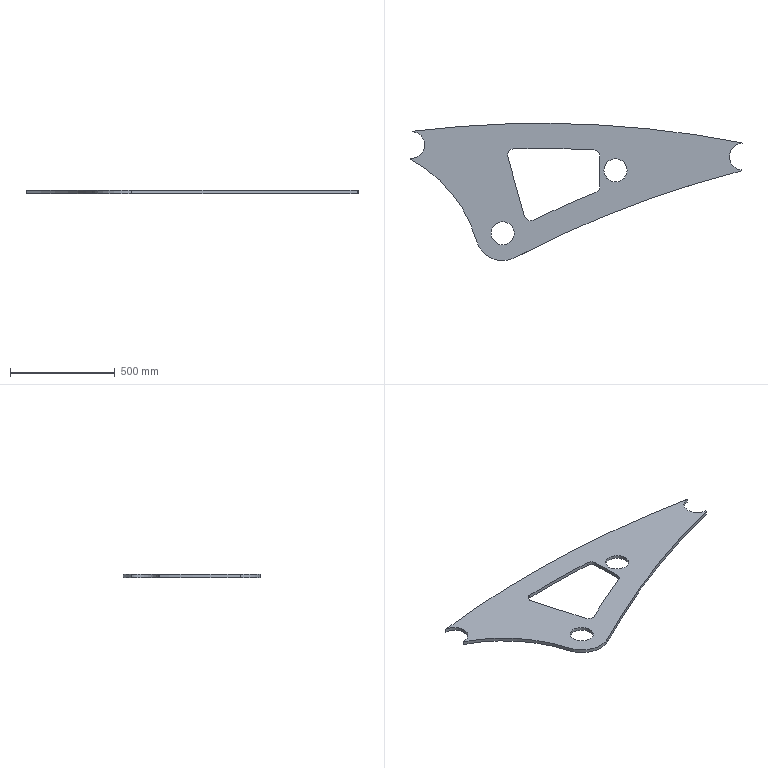Part | SolidWorks | features Extrusion 1 | 1 solid | 26 faces | box 1582 x 654.084 x 16 mm | volume 7594326 mm3 | cylinder 18 | plane 8 | commonest cylinder face diameters 60 x5 110 x4 128 x3 10000 x2 260 x1 1260 x1
STEP:
#1=CARTESIAN_POINT('',(52.281,402.337,16.));
#2=VERTEX_POINT('',#1);
#3=CARTESIAN_POINT('',(23.084,372.348,16.));
#4=VERTEX_POINT('',#3);
#5=CARTESIAN_POINT('',(53.084,372.348,16.));
#6=DIRECTION('',(0.,0.,1.));
#7=DIRECTION('',(-1.,0.,0.));
#8=AXIS2_PLACEMENT_3D('',#5,#6,#7);
#9=CIRCLE('',#8,30.);
#10=EDGE_CURVE('',#2,#4,#9,.T.);
#11=ORIENTED_EDGE('',*,*,#10,.T.);
#12=CARTESIAN_POINT('',(23.084,372.348,0.));
#13=VERTEX_POINT('',#12);
#14=CARTESIAN_POINT('',(23.084,372.348,16.));
#15=DIRECTION('',(0.,0.,-1.));
#16=VECTOR('',#15,1000.);
#17=LINE('',#14,#16);
#18=EDGE_CURVE('',#4,#13,#17,.T.);
#19=ORIENTED_EDGE('',*,*,#18,.T.);
#20=CARTESIAN_POINT('',(52.281,402.337,0.));
#21=VERTEX_POINT('',#20);
#22=CARTESIAN_POINT('',(53.084,372.348,0.));
#23=DIRECTION('',(0.,0.,1.));
#24=DIRECTION('',(-1.,0.,0.));
#25=AXIS2_PLACEMENT_3D('',#22,#23,#24);
#26=CIRCLE('',#25,30.);
#27=EDGE_CURVE('',#21,#13,#26,.T.);
#28=ORIENTED_EDGE('',*,*,#27,.F.);
#29=CARTESIAN_POINT('',(52.281,402.337,16.));
#30=DIRECTION('',(0.,0.,-1.));
#31=VECTOR('',#30,1000.);
#32=LINE('',#29,#31);
#33=EDGE_CURVE('',#2,#21,#32,.T.);
#34=ORIENTED_EDGE('',*,*,#33,.F.);
#35=EDGE_LOOP('',(#11,#19,#28,#34));
#36=FACE_OUTER_BOUND('',#35,.T.);
#37=CARTESIAN_POINT('',(53.084,372.348,16.));
#38=DIRECTION('',(0.,0.,-1.));
#39=DIRECTION('',(-1.,0.,0.));
#40=AXIS2_PLACEMENT_3D('',#37,#38,#39);
#41=CYLINDRICAL_SURFACE('',#40,30.);
#42=ADVANCED_FACE('',(#36),#41,.F.);
#43=CARTESIAN_POINT('',(483.,300.,16.));
#44=VERTEX_POINT('',#43);
#45=CARTESIAN_POINT('',(593.,300.,16.));
#46=VERTEX_POINT('',#45);
#47=CARTESIAN_POINT('',(538.,300.,16.));
#48=DIRECTION('',(0.,0.,1.));
#49=DIRECTION('',(1.,0.,0.));
#50=AXIS2_PLACEMENT_3D('',#47,#48,#49);
#51=CIRCLE('',#50,55.);
#52=EDGE_CURVE('',#44,#46,#51,.T.);
#53=ORIENTED_EDGE('',*,*,#52,.T.);
#54=CARTESIAN_POINT('',(593.,300.,0.));
#55=VERTEX_POINT('',#54);
#56=CARTESIAN_POINT('',(593.,300.,16.));
#57=DIRECTION('',(0.,0.,-1.));
#58=VECTOR('',#57,1000.);
#59=LINE('',#56,#58);
#60=EDGE_CURVE('',#46,#55,#59,.T.);
#61=ORIENTED_EDGE('',*,*,#60,.T.);
#62=CARTESIAN_POINT('',(483.,300.,0.));
#63=VERTEX_POINT('',#62);
#64=CARTESIAN_POINT('',(538.,300.,0.));
#65=DIRECTION('',(0.,0.,1.));
#66=DIRECTION('',(1.,0.,0.));
#67=AXIS2_PLACEMENT_3D('',#64,#65,#66);
#68=CIRCLE('',#67,55.);
#69=EDGE_CURVE('',#63,#55,#68,.T.);
#70=ORIENTED_EDGE('',*,*,#69,.F.);
#71=CARTESIAN_POINT('',(483.,300.,16.));
#72=DIRECTION('',(0.,0.,-1.));
#73=VECTOR('',#72,1000.);
#74=LINE('',#71,#73);
#75=EDGE_CURVE('',#44,#63,#74,.T.);
#76=ORIENTED_EDGE('',*,*,#75,.F.);
#77=EDGE_LOOP('',(#53,#61,#70,#76));
#78=FACE_OUTER_BOUND('',#77,.T.);
#79=CARTESIAN_POINT('',(538.,300.,16.));
#80=DIRECTION('',(0.,0.,-1.));
#81=DIRECTION('',(-1.,0.,0.));
#82=AXIS2_PLACEMENT_3D('',#79,#80,#81);
#83=CYLINDRICAL_SURFACE('',#82,55.);
#84=ADVANCED_FACE('',(#78),#83,.F.);
#85=CARTESIAN_POINT('',(-55.,0.,16.));
#86=VERTEX_POINT('',#85);
#87=CARTESIAN_POINT('',(55.,0.,16.));
#88=VERTEX_POINT('',#87);
#89=CARTESIAN_POINT('',(0.,0.,16.));
#90=DIRECTION('',(0.,0.,1.));
#91=DIRECTION('',(1.,0.,0.));
#92=AXIS2_PLACEMENT_3D('',#89,#90,#91);
#93=CIRCLE('',#92,55.);
#94=EDGE_CURVE('',#86,#88,#93,.T.);
#95=ORIENTED_EDGE('',*,*,#94,.T.);
#96=CARTESIAN_POINT('',(55.,0.,0.));
#97=VERTEX_POINT('',#96);
#98=CARTESIAN_POINT('',(55.,0.,16.));
#99=DIRECTION('',(0.,0.,-1.));
#100=VECTOR('',#99,1000.);
#101=LINE('',#98,#100);
#102=EDGE_CURVE('',#88,#97,#101,.T.);
#103=ORIENTED_EDGE('',*,*,#102,.T.);
#104=CARTESIAN_POINT('',(-55.,0.,0.));
#105=VERTEX_POINT('',#104);
#106=CARTESIAN_POINT('',(0.,0.,0.));
#107=DIRECTION('',(0.,0.,1.));
#108=DIRECTION('',(1.,0.,0.));
#109=AXIS2_PLACEMENT_3D('',#106,#107,#108);
#110=CIRCLE('',#109,55.);
#111=EDGE_CURVE('',#105,#97,#110,.T.);
#112=ORIENTED_EDGE('',*,*,#111,.F.);
#113=CARTESIAN_POINT('',(-55.,0.,16.));
#114=DIRECTION('',(0.,0.,-1.));
#115=VECTOR('',#114,1000.);
#116=LINE('',#113,#115);
#117=EDGE_CURVE('',#86,#105,#116,.T.);
#118=ORIENTED_EDGE('',*,*,#117,.F.);
#119=EDGE_LOOP('',(#95,#103,#112,#118));
#120=FACE_OUTER_BOUND('',#119,.T.);
#121=CARTESIAN_POINT('',(0.,0.,16.));
#122=DIRECTION('',(0.,0.,-1.));
#123=DIRECTION('',(-1.,0.,0.));
#124=AXIS2_PLACEMENT_3D('',#121,#122,#123);
#125=CYLINDRICAL_SURFACE('',#124,55.);
#126=ADVANCED_FACE('',(#120),#125,.F.);
#127=CARTESIAN_POINT('',(1080.5,365.5,16.));
#128=VERTEX_POINT('',#127);
#129=CARTESIAN_POINT('',(1140.709,429.388,16.));
#130=VERTEX_POINT('',#129);
#131=CARTESIAN_POINT('',(1144.5,365.5,16.));
#132=DIRECTION('',(0.,0.,-1.));
#133=DIRECTION('',(1.,0.,0.));
#134=AXIS2_PLACEMENT_3D('',#131,#132,#133);
#135=CIRCLE('',#134,64.);
#136=EDGE_CURVE('',#128,#130,#135,.T.);
#137=ORIENTED_EDGE('',*,*,#136,.F.);
#138=CARTESIAN_POINT('',(1080.5,365.5,0.));
#139=VERTEX_POINT('',#138);
#140=CARTESIAN_POINT('',(1080.5,365.5,16.));
#141=DIRECTION('',(0.,0.,-1.));
#142=VECTOR('',#141,1000.);
#143=LINE('',#140,#142);
#144=EDGE_CURVE('',#128,#139,#143,.T.);
#145=ORIENTED_EDGE('',*,*,#144,.T.);
#146=CARTESIAN_POINT('',(1140.709,429.388,0.));
#147=VERTEX_POINT('',#146);
#148=CARTESIAN_POINT('',(1144.5,365.5,0.));
#149=DIRECTION('',(0.,0.,-1.));
#150=DIRECTION('',(1.,0.,0.));
#151=AXIS2_PLACEMENT_3D('',#148,#149,#150);
#152=CIRCLE('',#151,64.);
#153=EDGE_CURVE('',#139,#147,#152,.T.);
#154=ORIENTED_EDGE('',*,*,#153,.T.);
#155=CARTESIAN_POINT('',(1140.709,429.388,16.));
#156=DIRECTION('',(0.,0.,-1.));
#157=VECTOR('',#156,1000.);
#158=LINE('',#155,#157);
#159=EDGE_CURVE('',#130,#147,#158,.T.);
#160=ORIENTED_EDGE('',*,*,#159,.F.);
#161=EDGE_LOOP('',(#137,#145,#154,#160));
#162=FACE_OUTER_BOUND('',#161,.T.);
#163=CARTESIAN_POINT('',(1144.5,365.5,16.));
#164=DIRECTION('',(0.,0.,-1.));
#165=DIRECTION('',(-1.,0.,0.));
#166=AXIS2_PLACEMENT_3D('',#163,#164,#165);
#167=CYLINDRICAL_SURFACE('',#166,64.);
#168=ADVANCED_FACE('',(#162),#167,.F.);
#169=ORIENTED_EDGE('',*,*,#52,.F.);
#170=CARTESIAN_POINT('',(538.,300.,16.));
#171=DIRECTION('',(0.,0.,1.));
#172=DIRECTION('',(1.,0.,0.));
#173=AXIS2_PLACEMENT_3D('',#170,#171,#172);
#174=CIRCLE('',#173,55.);
#175=EDGE_CURVE('',#46,#44,#174,.T.);
#176=ORIENTED_EDGE('',*,*,#175,.F.);
#177=EDGE_LOOP('',(#169,#176));
#178=FACE_BOUND('',#177,.T.);
#179=CARTESIAN_POINT('',(1140.523,431.512,16.));
#180=VERTEX_POINT('',#179);
#181=CARTESIAN_POINT('',(-429.795,486.409,16.));
#182=VERTEX_POINT('',#181);
#183=CARTESIAN_POINT('',(182.843,-4475.916,16.));
#184=DIRECTION('',(0.,0.,1.));
#185=DIRECTION('',(1.,0.,0.));
#186=AXIS2_PLACEMENT_3D('',#183,#184,#185);
#187=CIRCLE('',#186,5000.);
#188=EDGE_CURVE('',#180,#182,#187,.T.);
#189=ORIENTED_EDGE('',*,*,#188,.T.);
#190=CARTESIAN_POINT('',(-429.922,484.956,16.));
#191=VERTEX_POINT('',#190);
#192=CARTESIAN_POINT('',(-429.922,484.956,16.));
#193=DIRECTION('',(-0.08716,-0.9962,0.));
#194=VECTOR('',#193,1000.);
#195=LINE('',#192,#194);
#196=EDGE_CURVE('',#182,#191,#195,.T.);
#197=ORIENTED_EDGE('',*,*,#196,.T.);
#198=CARTESIAN_POINT('',(-441.078,357.444,16.));
#199=VERTEX_POINT('',#198);
#200=CARTESIAN_POINT('',(-435.5,421.2,16.));
#201=DIRECTION('',(0.,0.,-1.));
#202=DIRECTION('',(1.,0.,0.));
#203=AXIS2_PLACEMENT_3D('',#200,#201,#202);
#204=CIRCLE('',#203,64.);
#205=EDGE_CURVE('',#191,#199,#204,.T.);
#206=ORIENTED_EDGE('',*,*,#205,.T.);
#207=CARTESIAN_POINT('',(-441.487,352.773,16.));
#208=VERTEX_POINT('',#207);
#209=CARTESIAN_POINT('',(-441.487,352.773,16.));
#210=DIRECTION('',(-0.08716,-0.9962,0.));
#211=VECTOR('',#210,1000.);
#212=LINE('',#209,#211);
#213=EDGE_CURVE('',#199,#208,#212,.T.);
#214=ORIENTED_EDGE('',*,*,#213,.T.);
#215=CARTESIAN_POINT('',(-125.106,-35.333,16.));
#216=VERTEX_POINT('',#215);
#217=CARTESIAN_POINT('',(-731.391,-206.562,16.));
#218=DIRECTION('',(0.,0.,-1.));
#219=DIRECTION('',(1.,0.,0.));
#220=AXIS2_PLACEMENT_3D('',#217,#218,#219);
#221=CIRCLE('',#220,630.);
#222=EDGE_CURVE('',#208,#216,#221,.T.);
#223=ORIENTED_EDGE('',*,*,#222,.T.);
#224=CARTESIAN_POINT('',(60.222,-115.21,16.));
#225=VERTEX_POINT('',#224);
#226=CARTESIAN_POINT('',(0.,0.,16.));
#227=DIRECTION('',(0.,0.,1.));
#228=DIRECTION('',(1.,0.,0.));
#229=AXIS2_PLACEMENT_3D('',#226,#227,#228);
#230=CIRCLE('',#229,130.);
#231=EDGE_CURVE('',#216,#225,#230,.T.);
#232=ORIENTED_EDGE('',*,*,#231,.T.);
#233=CARTESIAN_POINT('',(1136.4,297.425,16.));
#234=VERTEX_POINT('',#233);
#235=CARTESIAN_POINT('',(2376.439,-4546.366,16.));
#236=DIRECTION('',(0.,0.,-1.));
#237=DIRECTION('',(1.,0.,0.));
#238=AXIS2_PLACEMENT_3D('',#235,#236,#237);
#239=CIRCLE('',#238,5000.);
#240=EDGE_CURVE('',#225,#234,#239,.T.);
#241=ORIENTED_EDGE('',*,*,#240,.T.);
#242=CARTESIAN_POINT('',(1135.994,302.068,16.));
#243=VERTEX_POINT('',#242);
#244=CARTESIAN_POINT('',(1135.994,302.068,16.));
#245=DIRECTION('',(-0.08716,0.9962,0.));
#246=VECTOR('',#245,1000.);
#247=LINE('',#244,#246);
#248=EDGE_CURVE('',#234,#243,#247,.T.);
#249=ORIENTED_EDGE('',*,*,#248,.T.);
#250=CARTESIAN_POINT('',(1144.5,365.5,16.));
#251=DIRECTION('',(0.,0.,-1.));
#252=DIRECTION('',(1.,0.,0.));
#253=AXIS2_PLACEMENT_3D('',#250,#251,#252);
#254=CIRCLE('',#253,64.);
#255=EDGE_CURVE('',#243,#128,#254,.T.);
#256=ORIENTED_EDGE('',*,*,#255,.T.);
#257=ORIENTED_EDGE('',*,*,#136,.T.);
#258=CARTESIAN_POINT('',(1140.709,429.388,16.));
#259=DIRECTION('',(-0.08716,0.9962,0.));
#260=VECTOR('',#259,1000.);
#261=LINE('',#258,#260);
#262=EDGE_CURVE('',#130,#180,#261,.T.);
#263=ORIENTED_EDGE('',*,*,#262,.T.);
#264=EDGE_LOOP('',(#189,#197,#206,#214,#223,#232,#241,#249,#256,#257,#263));
#265=FACE_OUTER_BOUND('',#264,.T.);
#266=ORIENTED_EDGE('',*,*,#94,.F.);
#267=CARTESIAN_POINT('',(0.,0.,16.));
#268=DIRECTION('',(0.,0.,1.));
#269=DIRECTION('',(1.,0.,0.));
#270=AXIS2_PLACEMENT_3D('',#267,#268,#269);
#271=CIRCLE('',#270,55.);
#272=EDGE_CURVE('',#88,#86,#271,.T.);
#273=ORIENTED_EDGE('',*,*,#272,.F.);
#274=EDGE_LOOP('',(#266,#273));
#275=FACE_BOUND('',#274,.T.);
#276=CARTESIAN_POINT('',(146.367,62.45,16.));
#277=VERTEX_POINT('',#276);
#278=CARTESIAN_POINT('',(444.321,195.082,16.));
#279=VERTEX_POINT('',#278);
#280=CARTESIAN_POINT('',(2376.439,-4546.366,16.));
#281=DIRECTION('',(0.,0.,-1.));
#282=DIRECTION('',(1.,0.,0.));
#283=AXIS2_PLACEMENT_3D('',#280,#281,#282);
#284=CIRCLE('',#283,5120.);
#285=EDGE_CURVE('',#277,#279,#284,.T.);
#286=ORIENTED_EDGE('',*,*,#285,.F.);
#287=CARTESIAN_POINT('',(104.438,81.271,16.));
#288=VERTEX_POINT('',#287);
#289=CARTESIAN_POINT('',(133.3,89.455,16.));
#290=DIRECTION('',(0.,0.,1.));
#291=DIRECTION('',(1.,0.,0.));
#292=AXIS2_PLACEMENT_3D('',#289,#290,#291);
#293=CIRCLE('',#292,30.);
#294=EDGE_CURVE('',#288,#277,#293,.T.);
#295=ORIENTED_EDGE('',*,*,#294,.F.);
#296=CARTESIAN_POINT('',(24.221,364.163,16.));
#297=VERTEX_POINT('',#296);
#298=CARTESIAN_POINT('',(104.438,81.271,16.));
#299=DIRECTION('',(0.2728,-0.9621,0.));
#300=VECTOR('',#299,1000.);
#301=LINE('',#298,#300);
#302=EDGE_CURVE('',#297,#288,#301,.T.);
#303=ORIENTED_EDGE('',*,*,#302,.F.);
#304=CARTESIAN_POINT('',(53.084,372.348,16.));
#305=DIRECTION('',(0.,0.,1.));
#306=DIRECTION('',(-1.,0.,0.));
#307=AXIS2_PLACEMENT_3D('',#304,#305,#306);
#308=CIRCLE('',#307,30.);
#309=EDGE_CURVE('',#4,#297,#308,.T.);
#310=ORIENTED_EDGE('',*,*,#309,.F.);
#311=ORIENTED_EDGE('',*,*,#10,.F.);
#312=CARTESIAN_POINT('',(434.547,397.588,16.));
#313=VERTEX_POINT('',#312);
#314=CARTESIAN_POINT('',(182.843,-4475.916,16.));
#315=DIRECTION('',(0.,0.,1.));
#316=DIRECTION('',(1.,0.,0.));
#317=AXIS2_PLACEMENT_3D('',#314,#315,#316);
#318=CIRCLE('',#317,4880.);
#319=EDGE_CURVE('',#313,#2,#318,.T.);
#320=ORIENTED_EDGE('',*,*,#319,.F.);
#321=CARTESIAN_POINT('',(463.,367.628,16.));
#322=VERTEX_POINT('',#321);
#323=CARTESIAN_POINT('',(433.,367.628,16.));
#324=DIRECTION('',(0.,0.,1.));
#325=DIRECTION('',(1.,0.,0.));
#326=AXIS2_PLACEMENT_3D('',#323,#324,#325);
#327=CIRCLE('',#326,30.);
#328=EDGE_CURVE('',#322,#313,#327,.T.);
#329=ORIENTED_EDGE('',*,*,#328,.F.);
#330=CARTESIAN_POINT('',(463.,222.864,16.));
#331=VERTEX_POINT('',#330);
#332=CARTESIAN_POINT('',(463.,367.628,16.));
#333=DIRECTION('',(0.,1.,0.));
#334=VECTOR('',#333,1000.);
#335=LINE('',#332,#334);
#336=EDGE_CURVE('',#331,#322,#335,.T.);
#337=ORIENTED_EDGE('',*,*,#336,.F.);
#338=CARTESIAN_POINT('',(433.,222.864,16.));
#339=DIRECTION('',(0.,0.,1.));
#340=DIRECTION('',(1.,0.,0.));
#341=AXIS2_PLACEMENT_3D('',#338,#339,#340);
#342=CIRCLE('',#341,30.);
#343=EDGE_CURVE('',#279,#331,#342,.T.);
#344=ORIENTED_EDGE('',*,*,#343,.F.);
#345=EDGE_LOOP('',(#286,#295,#303,#310,#311,#320,#329,#337,#344));
#346=FACE_BOUND('',#345,.T.);
#347=CARTESIAN_POINT('',(182.843,-4475.916,16.));
#348=DIRECTION('',(0.,0.,1.));
#349=DIRECTION('',(1.,0.,0.));
#350=AXIS2_PLACEMENT_3D('',#347,#348,#349);
#351=PLANE('',#350);
#352=ADVANCED_FACE('',(#178,#265,#275,#346),#351,.T.);
#353=ORIENTED_EDGE('',*,*,#69,.T.);
#354=CARTESIAN_POINT('',(538.,300.,0.));
#355=DIRECTION('',(0.,0.,1.));
#356=DIRECTION('',(1.,0.,0.));
#357=AXIS2_PLACEMENT_3D('',#354,#355,#356);
#358=CIRCLE('',#357,55.);
#359=EDGE_CURVE('',#55,#63,#358,.T.);
#360=ORIENTED_EDGE('',*,*,#359,.T.);
#361=EDGE_LOOP('',(#353,#360));
#362=FACE_BOUND('',#361,.T.);
#363=CARTESIAN_POINT('',(1140.523,431.512,0.));
#364=VERTEX_POINT('',#363);
#365=CARTESIAN_POINT('',(-429.795,486.409,0.));
#366=VERTEX_POINT('',#365);
#367=CARTESIAN_POINT('',(182.843,-4475.916,0.));
#368=DIRECTION('',(0.,0.,1.));
#369=DIRECTION('',(1.,0.,0.));
#370=AXIS2_PLACEMENT_3D('',#367,#368,#369);
#371=CIRCLE('',#370,5000.);
#372=EDGE_CURVE('',#364,#366,#371,.T.);
#373=ORIENTED_EDGE('',*,*,#372,.F.);
#374=CARTESIAN_POINT('',(1140.709,429.388,0.));
#375=DIRECTION('',(-0.08716,0.9962,0.));
#376=VECTOR('',#375,1000.);
#377=LINE('',#374,#376);
#378=EDGE_CURVE('',#147,#364,#377,.T.);
#379=ORIENTED_EDGE('',*,*,#378,.F.);
#380=ORIENTED_EDGE('',*,*,#153,.F.);
#381=CARTESIAN_POINT('',(1135.994,302.068,0.));
#382=VERTEX_POINT('',#381);
#383=CARTESIAN_POINT('',(1144.5,365.5,0.));
#384=DIRECTION('',(0.,0.,-1.));
#385=DIRECTION('',(1.,0.,0.));
#386=AXIS2_PLACEMENT_3D('',#383,#384,#385);
#387=CIRCLE('',#386,64.);
#388=EDGE_CURVE('',#382,#139,#387,.T.);
#389=ORIENTED_EDGE('',*,*,#388,.F.);
#390=CARTESIAN_POINT('',(1136.4,297.425,0.));
#391=VERTEX_POINT('',#390);
#392=CARTESIAN_POINT('',(1135.994,302.068,0.));
#393=DIRECTION('',(-0.08716,0.9962,0.));
#394=VECTOR('',#393,1000.);
#395=LINE('',#392,#394);
#396=EDGE_CURVE('',#391,#382,#395,.T.);
#397=ORIENTED_EDGE('',*,*,#396,.F.);
#398=CARTESIAN_POINT('',(60.222,-115.21,0.));
#399=VERTEX_POINT('',#398);
#400=CARTESIAN_POINT('',(2376.439,-4546.366,0.));
#401=DIRECTION('',(0.,0.,-1.));
#402=DIRECTION('',(1.,0.,0.));
#403=AXIS2_PLACEMENT_3D('',#400,#401,#402);
#404=CIRCLE('',#403,5000.);
#405=EDGE_CURVE('',#399,#391,#404,.T.);
#406=ORIENTED_EDGE('',*,*,#405,.F.);
#407=CARTESIAN_POINT('',(-125.106,-35.333,0.));
#408=VERTEX_POINT('',#407);
#409=CARTESIAN_POINT('',(0.,0.,0.));
#410=DIRECTION('',(0.,0.,1.));
#411=DIRECTION('',(1.,0.,0.));
#412=AXIS2_PLACEMENT_3D('',#409,#410,#411);
#413=CIRCLE('',#412,130.);
#414=EDGE_CURVE('',#408,#399,#413,.T.);
#415=ORIENTED_EDGE('',*,*,#414,.F.);
#416=CARTESIAN_POINT('',(-441.487,352.773,0.));
#417=VERTEX_POINT('',#416);
#418=CARTESIAN_POINT('',(-731.391,-206.562,0.));
#419=DIRECTION('',(0.,0.,-1.));
#420=DIRECTION('',(1.,0.,0.));
#421=AXIS2_PLACEMENT_3D('',#418,#419,#420);
#422=CIRCLE('',#421,630.);
#423=EDGE_CURVE('',#417,#408,#422,.T.);
#424=ORIENTED_EDGE('',*,*,#423,.F.);
#425=CARTESIAN_POINT('',(-441.078,357.444,0.));
#426=VERTEX_POINT('',#425);
#427=CARTESIAN_POINT('',(-441.487,352.773,0.));
#428=DIRECTION('',(-0.08716,-0.9962,0.));
#429=VECTOR('',#428,1000.);
#430=LINE('',#427,#429);
#431=EDGE_CURVE('',#426,#417,#430,.T.);
#432=ORIENTED_EDGE('',*,*,#431,.F.);
#433=CARTESIAN_POINT('',(-429.922,484.956,0.));
#434=VERTEX_POINT('',#433);
#435=CARTESIAN_POINT('',(-435.5,421.2,0.));
#436=DIRECTION('',(0.,0.,-1.));
#437=DIRECTION('',(1.,0.,0.));
#438=AXIS2_PLACEMENT_3D('',#435,#436,#437);
#439=CIRCLE('',#438,64.);
#440=EDGE_CURVE('',#434,#426,#439,.T.);
#441=ORIENTED_EDGE('',*,*,#440,.F.);
#442=CARTESIAN_POINT('',(-429.922,484.956,0.));
#443=DIRECTION('',(-0.08716,-0.9962,0.));
#444=VECTOR('',#443,1000.);
#445=LINE('',#442,#444);
#446=EDGE_CURVE('',#366,#434,#445,.T.);
#447=ORIENTED_EDGE('',*,*,#446,.F.);
#448=EDGE_LOOP('',(#373,#379,#380,#389,#397,#406,#415,#424,#432,#441,#447));
#449=FACE_OUTER_BOUND('',#448,.T.);
#450=ORIENTED_EDGE('',*,*,#111,.T.);
#451=CARTESIAN_POINT('',(0.,0.,0.));
#452=DIRECTION('',(0.,0.,1.));
#453=DIRECTION('',(1.,0.,0.));
#454=AXIS2_PLACEMENT_3D('',#451,#452,#453);
#455=CIRCLE('',#454,55.);
#456=EDGE_CURVE('',#97,#105,#455,.T.);
#457=ORIENTED_EDGE('',*,*,#456,.T.);
#458=EDGE_LOOP('',(#450,#457));
#459=FACE_BOUND('',#458,.T.);
#460=CARTESIAN_POINT('',(104.438,81.271,0.));
#461=VERTEX_POINT('',#460);
#462=CARTESIAN_POINT('',(146.367,62.45,0.));
#463=VERTEX_POINT('',#462);
#464=CARTESIAN_POINT('',(133.3,89.455,0.));
#465=DIRECTION('',(0.,0.,1.));
#466=DIRECTION('',(1.,0.,0.));
#467=AXIS2_PLACEMENT_3D('',#464,#465,#466);
#468=CIRCLE('',#467,30.);
#469=EDGE_CURVE('',#461,#463,#468,.T.);
#470=ORIENTED_EDGE('',*,*,#469,.T.);
#471=CARTESIAN_POINT('',(444.321,195.082,0.));
#472=VERTEX_POINT('',#471);
#473=CARTESIAN_POINT('',(2376.439,-4546.366,0.));
#474=DIRECTION('',(0.,0.,-1.));
#475=DIRECTION('',(1.,0.,0.));
#476=AXIS2_PLACEMENT_3D('',#473,#474,#475);
#477=CIRCLE('',#476,5120.);
#478=EDGE_CURVE('',#463,#472,#477,.T.);
#479=ORIENTED_EDGE('',*,*,#478,.T.);
#480=CARTESIAN_POINT('',(463.,222.864,0.));
#481=VERTEX_POINT('',#480);
#482=CARTESIAN_POINT('',(433.,222.864,0.));
#483=DIRECTION('',(0.,0.,1.));
#484=DIRECTION('',(1.,0.,0.));
#485=AXIS2_PLACEMENT_3D('',#482,#483,#484);
#486=CIRCLE('',#485,30.);
#487=EDGE_CURVE('',#472,#481,#486,.T.);
#488=ORIENTED_EDGE('',*,*,#487,.T.);
#489=CARTESIAN_POINT('',(463.,367.628,0.));
#490=VERTEX_POINT('',#489);
#491=CARTESIAN_POINT('',(463.,367.628,0.));
#492=DIRECTION('',(0.,1.,0.));
#493=VECTOR('',#492,1000.);
#494=LINE('',#491,#493);
#495=EDGE_CURVE('',#481,#490,#494,.T.);
#496=ORIENTED_EDGE('',*,*,#495,.T.);
#497=CARTESIAN_POINT('',(434.547,397.588,0.));
#498=VERTEX_POINT('',#497);
#499=CARTESIAN_POINT('',(433.,367.628,0.));
#500=DIRECTION('',(0.,0.,1.));
#501=DIRECTION('',(1.,0.,0.));
#502=AXIS2_PLACEMENT_3D('',#499,#500,#501);
#503=CIRCLE('',#502,30.);
#504=EDGE_CURVE('',#490,#498,#503,.T.);
#505=ORIENTED_EDGE('',*,*,#504,.T.);
#506=CARTESIAN_POINT('',(182.843,-4475.916,0.));
#507=DIRECTION('',(0.,0.,1.));
#508=DIRECTION('',(1.,0.,0.));
#509=AXIS2_PLACEMENT_3D('',#506,#507,#508);
#510=CIRCLE('',#509,4880.);
#511=EDGE_CURVE('',#498,#21,#510,.T.);
#512=ORIENTED_EDGE('',*,*,#511,.T.);
#513=ORIENTED_EDGE('',*,*,#27,.T.);
#514=CARTESIAN_POINT('',(24.221,364.163,0.));
#515=VERTEX_POINT('',#514);
#516=CARTESIAN_POINT('',(53.084,372.348,0.));
#517=DIRECTION('',(0.,0.,1.));
#518=DIRECTION('',(-1.,0.,0.));
#519=AXIS2_PLACEMENT_3D('',#516,#517,#518);
#520=CIRCLE('',#519,30.);
#521=EDGE_CURVE('',#13,#515,#520,.T.);
#522=ORIENTED_EDGE('',*,*,#521,.T.);
#523=CARTESIAN_POINT('',(104.438,81.271,0.));
#524=DIRECTION('',(0.2728,-0.9621,0.));
#525=VECTOR('',#524,1000.);
#526=LINE('',#523,#525);
#527=EDGE_CURVE('',#515,#461,#526,.T.);
#528=ORIENTED_EDGE('',*,*,#527,.T.);
#529=EDGE_LOOP('',(#470,#479,#488,#496,#505,#512,#513,#522,#528));
#530=FACE_BOUND('',#529,.T.);
#531=CARTESIAN_POINT('',(182.843,-4475.916,0.));
#532=DIRECTION('',(0.,0.,1.));
#533=DIRECTION('',(1.,0.,0.));
#534=AXIS2_PLACEMENT_3D('',#531,#532,#533);
#535=PLANE('',#534);
#536=ADVANCED_FACE('',(#362,#449,#459,#530),#535,.F.);
#537=ORIENTED_EDGE('',*,*,#372,.T.);
#538=CARTESIAN_POINT('',(-429.795,486.409,16.));
#539=DIRECTION('',(0.,0.,-1.));
#540=VECTOR('',#539,1000.);
#541=LINE('',#538,#540);
#542=EDGE_CURVE('',#182,#366,#541,.T.);
#543=ORIENTED_EDGE('',*,*,#542,.F.);
#544=ORIENTED_EDGE('',*,*,#188,.F.);
#545=CARTESIAN_POINT('',(1140.523,431.512,16.));
#546=DIRECTION('',(0.,0.,-1.));
#547=VECTOR('',#546,1000.);
#548=LINE('',#545,#547);
#549=EDGE_CURVE('',#180,#364,#548,.T.);
#550=ORIENTED_EDGE('',*,*,#549,.T.);
#551=EDGE_LOOP('',(#537,#543,#544,#550));
#552=FACE_OUTER_BOUND('',#551,.T.);
#553=CARTESIAN_POINT('',(182.843,-4475.916,16.));
#554=DIRECTION('',(0.,0.,-1.));
#555=DIRECTION('',(-1.,0.,0.));
#556=AXIS2_PLACEMENT_3D('',#553,#554,#555);
#557=CYLINDRICAL_SURFACE('',#556,5000.);
#558=ADVANCED_FACE('',(#552),#557,.T.);
#559=ORIENTED_EDGE('',*,*,#446,.T.);
#560=CARTESIAN_POINT('',(-429.922,484.956,16.));
#561=DIRECTION('',(0.,0.,-1.));
#562=VECTOR('',#561,1000.);
#563=LINE('',#560,#562);
#564=EDGE_CURVE('',#191,#434,#563,.T.);
#565=ORIENTED_EDGE('',*,*,#564,.F.);
#566=ORIENTED_EDGE('',*,*,#196,.F.);
#567=ORIENTED_EDGE('',*,*,#542,.T.);
#568=EDGE_LOOP('',(#559,#565,#566,#567));
#569=FACE_OUTER_BOUND('',#568,.T.);
#570=CARTESIAN_POINT('',(-429.922,484.956,16.));
#571=DIRECTION('',(0.9962,-0.08716,0.));
#572=DIRECTION('',(0.08716,0.9962,0.));
#573=AXIS2_PLACEMENT_3D('',#570,#571,#572);
#574=PLANE('',#573);
#575=ADVANCED_FACE('',(#569),#574,.F.);
#576=ORIENTED_EDGE('',*,*,#440,.T.);
#577=CARTESIAN_POINT('',(-441.078,357.444,16.));
#578=DIRECTION('',(0.,0.,-1.));
#579=VECTOR('',#578,1000.);
#580=LINE('',#577,#579);
#581=EDGE_CURVE('',#199,#426,#580,.T.);
#582=ORIENTED_EDGE('',*,*,#581,.F.);
#583=ORIENTED_EDGE('',*,*,#205,.F.);
#584=ORIENTED_EDGE('',*,*,#564,.T.);
#585=EDGE_LOOP('',(#576,#582,#583,#584));
#586=FACE_OUTER_BOUND('',#585,.T.);
#587=CARTESIAN_POINT('',(-435.5,421.2,16.));
#588=DIRECTION('',(0.,0.,-1.));
#589=DIRECTION('',(-1.,0.,0.));
#590=AXIS2_PLACEMENT_3D('',#587,#588,#589);
#591=CYLINDRICAL_SURFACE('',#590,64.);
#592=ADVANCED_FACE('',(#586),#591,.F.);
#593=ORIENTED_EDGE('',*,*,#431,.T.);
#594=CARTESIAN_POINT('',(-441.487,352.773,16.));
#595=DIRECTION('',(0.,0.,-1.));
#596=VECTOR('',#595,1000.);
#597=LINE('',#594,#596);
#598=EDGE_CURVE('',#208,#417,#597,.T.);
#599=ORIENTED_EDGE('',*,*,#598,.F.);
#600=ORIENTED_EDGE('',*,*,#213,.F.);
#601=ORIENTED_EDGE('',*,*,#581,.T.);
#602=EDGE_LOOP('',(#593,#599,#600,#601));
#603=FACE_OUTER_BOUND('',#602,.T.);
#604=CARTESIAN_POINT('',(-441.487,352.773,16.));
#605=DIRECTION('',(0.9962,-0.08716,0.));
#606=DIRECTION('',(0.08716,0.9962,0.));
#607=AXIS2_PLACEMENT_3D('',#604,#605,#606);
#608=PLANE('',#607);
#609=ADVANCED_FACE('',(#603),#608,.F.);
#610=ORIENTED_EDGE('',*,*,#423,.T.);
#611=CARTESIAN_POINT('',(-125.106,-35.333,16.));
#612=DIRECTION('',(0.,0.,-1.));
#613=VECTOR('',#612,1000.);
#614=LINE('',#611,#613);
#615=EDGE_CURVE('',#216,#408,#614,.T.);
#616=ORIENTED_EDGE('',*,*,#615,.F.);
#617=ORIENTED_EDGE('',*,*,#222,.F.);
#618=ORIENTED_EDGE('',*,*,#598,.T.);
#619=EDGE_LOOP('',(#610,#616,#617,#618));
#620=FACE_OUTER_BOUND('',#619,.T.);
#621=CARTESIAN_POINT('',(-731.391,-206.562,16.));
#622=DIRECTION('',(0.,0.,-1.));
#623=DIRECTION('',(-1.,0.,0.));
#624=AXIS2_PLACEMENT_3D('',#621,#622,#623);
#625=CYLINDRICAL_SURFACE('',#624,630.);
#626=ADVANCED_FACE('',(#620),#625,.F.);
#627=ORIENTED_EDGE('',*,*,#414,.T.);
#628=CARTESIAN_POINT('',(60.222,-115.21,16.));
#629=DIRECTION('',(0.,0.,-1.));
#630=VECTOR('',#629,1000.);
#631=LINE('',#628,#630);
#632=EDGE_CURVE('',#225,#399,#631,.T.);
#633=ORIENTED_EDGE('',*,*,#632,.F.);
#634=ORIENTED_EDGE('',*,*,#231,.F.);
#635=ORIENTED_EDGE('',*,*,#615,.T.);
#636=EDGE_LOOP('',(#627,#633,#634,#635));
#637=FACE_OUTER_BOUND('',#636,.T.);
#638=CARTESIAN_POINT('',(0.,0.,16.));
#639=DIRECTION('',(0.,0.,-1.));
#640=DIRECTION('',(-1.,0.,0.));
#641=AXIS2_PLACEMENT_3D('',#638,#639,#640);
#642=CYLINDRICAL_SURFACE('',#641,130.);
#643=ADVANCED_FACE('',(#637),#642,.T.);
#644=ORIENTED_EDGE('',*,*,#405,.T.);
#645=CARTESIAN_POINT('',(1136.4,297.425,16.));
#646=DIRECTION('',(0.,0.,-1.));
#647=VECTOR('',#646,1000.);
#648=LINE('',#645,#647);
#649=EDGE_CURVE('',#234,#391,#648,.T.);
#650=ORIENTED_EDGE('',*,*,#649,.F.);
#651=ORIENTED_EDGE('',*,*,#240,.F.);
#652=ORIENTED_EDGE('',*,*,#632,.T.);
#653=EDGE_LOOP('',(#644,#650,#651,#652));
#654=FACE_OUTER_BOUND('',#653,.T.);
#655=CARTESIAN_POINT('',(2376.439,-4546.366,16.));
#656=DIRECTION('',(0.,0.,-1.));
#657=DIRECTION('',(-1.,0.,0.));
#658=AXIS2_PLACEMENT_3D('',#655,#656,#657);
#659=CYLINDRICAL_SURFACE('',#658,5000.);
#660=ADVANCED_FACE('',(#654),#659,.F.);
#661=ORIENTED_EDGE('',*,*,#396,.T.);
#662=CARTESIAN_POINT('',(1135.994,302.068,16.));
#663=DIRECTION('',(0.,0.,-1.));
#664=VECTOR('',#663,1000.);
#665=LINE('',#662,#664);
#666=EDGE_CURVE('',#243,#382,#665,.T.);
#667=ORIENTED_EDGE('',*,*,#666,.F.);
#668=ORIENTED_EDGE('',*,*,#248,.F.);
#669=ORIENTED_EDGE('',*,*,#649,.T.);
#670=EDGE_LOOP('',(#661,#667,#668,#669));
#671=FACE_OUTER_BOUND('',#670,.T.);
#672=CARTESIAN_POINT('',(1135.994,302.068,16.));
#673=DIRECTION('',(-0.9962,-0.08716,0.));
#674=DIRECTION('',(0.08716,-0.9962,0.));
#675=AXIS2_PLACEMENT_3D('',#672,#673,#674);
#676=PLANE('',#675);
#677=ADVANCED_FACE('',(#671),#676,.F.);
#678=ORIENTED_EDGE('',*,*,#144,.F.);
#679=ORIENTED_EDGE('',*,*,#255,.F.);
#680=ORIENTED_EDGE('',*,*,#666,.T.);
#681=ORIENTED_EDGE('',*,*,#388,.T.);
#682=EDGE_LOOP('',(#678,#679,#680,#681));
#683=FACE_OUTER_BOUND('',#682,.T.);
#684=CARTESIAN_POINT('',(1144.5,365.5,16.));
#685=DIRECTION('',(0.,0.,-1.));
#686=DIRECTION('',(-1.,0.,0.));
#687=AXIS2_PLACEMENT_3D('',#684,#685,#686);
#688=CYLINDRICAL_SURFACE('',#687,64.);
#689=ADVANCED_FACE('',(#683),#688,.F.);
#690=ORIENTED_EDGE('',*,*,#378,.T.);
#691=ORIENTED_EDGE('',*,*,#549,.F.);
#692=ORIENTED_EDGE('',*,*,#262,.F.);
#693=ORIENTED_EDGE('',*,*,#159,.T.);
#694=EDGE_LOOP('',(#690,#691,#692,#693));
#695=FACE_OUTER_BOUND('',#694,.T.);
#696=CARTESIAN_POINT('',(1140.709,429.388,16.));
#697=DIRECTION('',(-0.9962,-0.08716,0.));
#698=DIRECTION('',(0.08716,-0.9962,0.));
#699=AXIS2_PLACEMENT_3D('',#696,#697,#698);
#700=PLANE('',#699);
#701=ADVANCED_FACE('',(#695),#700,.F.);
#702=ORIENTED_EDGE('',*,*,#102,.F.);
#703=ORIENTED_EDGE('',*,*,#272,.T.);
#704=ORIENTED_EDGE('',*,*,#117,.T.);
#705=ORIENTED_EDGE('',*,*,#456,.F.);
#706=EDGE_LOOP('',(#702,#703,#704,#705));
#707=FACE_OUTER_BOUND('',#706,.T.);
#708=CARTESIAN_POINT('',(0.,0.,16.));
#709=DIRECTION('',(0.,0.,-1.));
#710=DIRECTION('',(-1.,0.,0.));
#711=AXIS2_PLACEMENT_3D('',#708,#709,#710);
#712=CYLINDRICAL_SURFACE('',#711,55.);
#713=ADVANCED_FACE('',(#707),#712,.F.);
#714=ORIENTED_EDGE('',*,*,#60,.F.);
#715=ORIENTED_EDGE('',*,*,#175,.T.);
#716=ORIENTED_EDGE('',*,*,#75,.T.);
#717=ORIENTED_EDGE('',*,*,#359,.F.);
#718=EDGE_LOOP('',(#714,#715,#716,#717));
#719=FACE_OUTER_BOUND('',#718,.T.);
#720=CARTESIAN_POINT('',(538.,300.,16.));
#721=DIRECTION('',(0.,0.,-1.));
#722=DIRECTION('',(-1.,0.,0.));
#723=AXIS2_PLACEMENT_3D('',#720,#721,#722);
#724=CYLINDRICAL_SURFACE('',#723,55.);
#725=ADVANCED_FACE('',(#719),#724,.F.);
#726=ORIENTED_EDGE('',*,*,#469,.F.);
#727=CARTESIAN_POINT('',(104.438,81.271,16.));
#728=DIRECTION('',(0.,0.,-1.));
#729=VECTOR('',#728,1000.);
#730=LINE('',#727,#729);
#731=EDGE_CURVE('',#288,#461,#730,.T.);
#732=ORIENTED_EDGE('',*,*,#731,.F.);
#733=ORIENTED_EDGE('',*,*,#294,.T.);
#734=CARTESIAN_POINT('',(146.367,62.45,16.));
#735=DIRECTION('',(0.,0.,-1.));
#736=VECTOR('',#735,1000.);
#737=LINE('',#734,#736);
#738=EDGE_CURVE('',#277,#463,#737,.T.);
#739=ORIENTED_EDGE('',*,*,#738,.T.);
#740=EDGE_LOOP('',(#726,#732,#733,#739));
#741=FACE_OUTER_BOUND('',#740,.T.);
#742=CARTESIAN_POINT('',(133.3,89.455,16.));
#743=DIRECTION('',(0.,0.,-1.));
#744=DIRECTION('',(-1.,0.,0.));
#745=AXIS2_PLACEMENT_3D('',#742,#743,#744);
#746=CYLINDRICAL_SURFACE('',#745,30.);
#747=ADVANCED_FACE('',(#741),#746,.F.);
#748=ORIENTED_EDGE('',*,*,#478,.F.);
#749=ORIENTED_EDGE('',*,*,#738,.F.);
#750=ORIENTED_EDGE('',*,*,#285,.T.);
#751=CARTESIAN_POINT('',(444.321,195.082,16.));
#752=DIRECTION('',(0.,0.,-1.));
#753=VECTOR('',#752,1000.);
#754=LINE('',#751,#753);
#755=EDGE_CURVE('',#279,#472,#754,.T.);
#756=ORIENTED_EDGE('',*,*,#755,.T.);
#757=EDGE_LOOP('',(#748,#749,#750,#756));
#758=FACE_OUTER_BOUND('',#757,.T.);
#759=CARTESIAN_POINT('',(2376.439,-4546.366,16.));
#760=DIRECTION('',(0.,0.,-1.));
#761=DIRECTION('',(-1.,0.,0.));
#762=AXIS2_PLACEMENT_3D('',#759,#760,#761);
#763=CYLINDRICAL_SURFACE('',#762,5120.);
#764=ADVANCED_FACE('',(#758),#763,.T.);
#765=ORIENTED_EDGE('',*,*,#487,.F.);
#766=ORIENTED_EDGE('',*,*,#755,.F.);
#767=ORIENTED_EDGE('',*,*,#343,.T.);
#768=CARTESIAN_POINT('',(463.,222.864,16.));
#769=DIRECTION('',(0.,0.,-1.));
#770=VECTOR('',#769,1000.);
#771=LINE('',#768,#770);
#772=EDGE_CURVE('',#331,#481,#771,.T.);
#773=ORIENTED_EDGE('',*,*,#772,.T.);
#774=EDGE_LOOP('',(#765,#766,#767,#773));
#775=FACE_OUTER_BOUND('',#774,.T.);
#776=CARTESIAN_POINT('',(433.,222.864,16.));
#777=DIRECTION('',(0.,0.,-1.));
#778=DIRECTION('',(-1.,0.,0.));
#779=AXIS2_PLACEMENT_3D('',#776,#777,#778);
#780=CYLINDRICAL_SURFACE('',#779,30.);
#781=ADVANCED_FACE('',(#775),#780,.F.);
#782=ORIENTED_EDGE('',*,*,#495,.F.);
#783=ORIENTED_EDGE('',*,*,#772,.F.);
#784=ORIENTED_EDGE('',*,*,#336,.T.);
#785=CARTESIAN_POINT('',(463.,367.628,16.));
#786=DIRECTION('',(0.,0.,-1.));
#787=VECTOR('',#786,1000.);
#788=LINE('',#785,#787);
#789=EDGE_CURVE('',#322,#490,#788,.T.);
#790=ORIENTED_EDGE('',*,*,#789,.T.);
#791=EDGE_LOOP('',(#782,#783,#784,#790));
#792=FACE_OUTER_BOUND('',#791,.T.);
#793=CARTESIAN_POINT('',(463.,367.628,16.));
#794=DIRECTION('',(-1.,0.,0.));
#795=DIRECTION('',(0.,-1.,0.));
#796=AXIS2_PLACEMENT_3D('',#793,#794,#795);
#797=PLANE('',#796);
#798=ADVANCED_FACE('',(#792),#797,.T.);
#799=ORIENTED_EDGE('',*,*,#504,.F.);
#800=ORIENTED_EDGE('',*,*,#789,.F.);
#801=ORIENTED_EDGE('',*,*,#328,.T.);
#802=CARTESIAN_POINT('',(434.547,397.588,16.));
#803=DIRECTION('',(0.,0.,-1.));
#804=VECTOR('',#803,1000.);
#805=LINE('',#802,#804);
#806=EDGE_CURVE('',#313,#498,#805,.T.);
#807=ORIENTED_EDGE('',*,*,#806,.T.);
#808=EDGE_LOOP('',(#799,#800,#801,#807));
#809=FACE_OUTER_BOUND('',#808,.T.);
#810=CARTESIAN_POINT('',(433.,367.628,16.));
#811=DIRECTION('',(0.,0.,-1.));
#812=DIRECTION('',(-1.,0.,0.));
#813=AXIS2_PLACEMENT_3D('',#810,#811,#812);
#814=CYLINDRICAL_SURFACE('',#813,30.);
#815=ADVANCED_FACE('',(#809),#814,.F.);
#816=ORIENTED_EDGE('',*,*,#511,.F.);
#817=ORIENTED_EDGE('',*,*,#806,.F.);
#818=ORIENTED_EDGE('',*,*,#319,.T.);
#819=ORIENTED_EDGE('',*,*,#33,.T.);
#820=EDGE_LOOP('',(#816,#817,#818,#819));
#821=FACE_OUTER_BOUND('',#820,.T.);
#822=CARTESIAN_POINT('',(182.843,-4475.916,16.));
#823=DIRECTION('',(0.,0.,-1.));
#824=DIRECTION('',(-1.,0.,0.));
#825=AXIS2_PLACEMENT_3D('',#822,#823,#824);
#826=CYLINDRICAL_SURFACE('',#825,4880.);
#827=ADVANCED_FACE('',(#821),#826,.F.);
#828=ORIENTED_EDGE('',*,*,#18,.F.);
#829=ORIENTED_EDGE('',*,*,#309,.T.);
#830=CARTESIAN_POINT('',(24.221,364.163,16.));
#831=DIRECTION('',(0.,0.,-1.));
#832=VECTOR('',#831,1000.);
#833=LINE('',#830,#832);
#834=EDGE_CURVE('',#297,#515,#833,.T.);
#835=ORIENTED_EDGE('',*,*,#834,.T.);
#836=ORIENTED_EDGE('',*,*,#521,.F.);
#837=EDGE_LOOP('',(#828,#829,#835,#836));
#838=FACE_OUTER_BOUND('',#837,.T.);
#839=CARTESIAN_POINT('',(53.084,372.348,16.));
#840=DIRECTION('',(0.,0.,-1.));
#841=DIRECTION('',(-1.,0.,0.));
#842=AXIS2_PLACEMENT_3D('',#839,#840,#841);
#843=CYLINDRICAL_SURFACE('',#842,30.);
#844=ADVANCED_FACE('',(#838),#843,.F.);
#845=ORIENTED_EDGE('',*,*,#527,.F.);
#846=ORIENTED_EDGE('',*,*,#834,.F.);
#847=ORIENTED_EDGE('',*,*,#302,.T.);
#848=ORIENTED_EDGE('',*,*,#731,.T.);
#849=EDGE_LOOP('',(#845,#846,#847,#848));
#850=FACE_OUTER_BOUND('',#849,.T.);
#851=CARTESIAN_POINT('',(104.438,81.271,16.));
#852=DIRECTION('',(0.9621,0.2728,0.));
#853=DIRECTION('',(-0.2728,0.9621,0.));
#854=AXIS2_PLACEMENT_3D('',#851,#852,#853);
#855=PLANE('',#854);
#856=ADVANCED_FACE('',(#850),#855,.T.);
#857=CLOSED_SHELL('',(#42,#84,#126,#168,#352,#536,#558,#575,#592,#609,#626,#643,#660,#677,#689,#701,#713,#725,#747,#764,#781,#798,#815,#827,#844,#856));
#858=MANIFOLD_SOLID_BREP('',#857);
#859=CARTESIAN_POINT('',(0.,0.,0.));
#860=DIRECTION('',(0.,0.,1.));
#861=DIRECTION('',(1.,0.,0.));
#862=AXIS2_PLACEMENT_3D('',#859,#860,#861);
#863=(LENGTH_UNIT()NAMED_UNIT(*)SI_UNIT(.MILLI.,.METRE.));
#864=UNCERTAINTY_MEASURE_WITH_UNIT(LENGTH_MEASURE(0.00001),#863,'','');
#865=(NAMED_UNIT(*)PLANE_ANGLE_UNIT()SI_UNIT($,.RADIAN.));
#866=(NAMED_UNIT(*)SI_UNIT($,.STERADIAN.)SOLID_ANGLE_UNIT());
#867=(GEOMETRIC_REPRESENTATION_CONTEXT(3)GLOBAL_UNCERTAINTY_ASSIGNED_CONTEXT((#864))GLOBAL_UNIT_ASSIGNED_CONTEXT((#863,#865,#866))REPRESENTATION_CONTEXT('',''));
#868=ADVANCED_BREP_SHAPE_REPRESENTATION('',(#858,#862),#867);